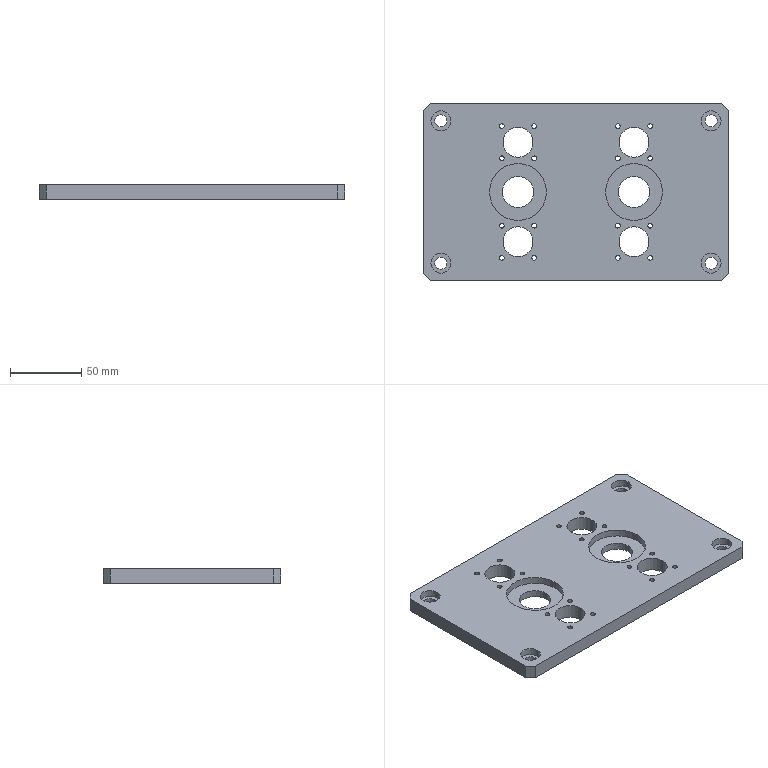Part | 1 solid | 80 faces | box 215 x 125 x 10 mm | volume 232446 mm3 | cylinder 64 | plane 16 | commonest cylinder face diameters 3.3 x32 8.5 x8 14 x8 21 x8 22 x4 40 x4